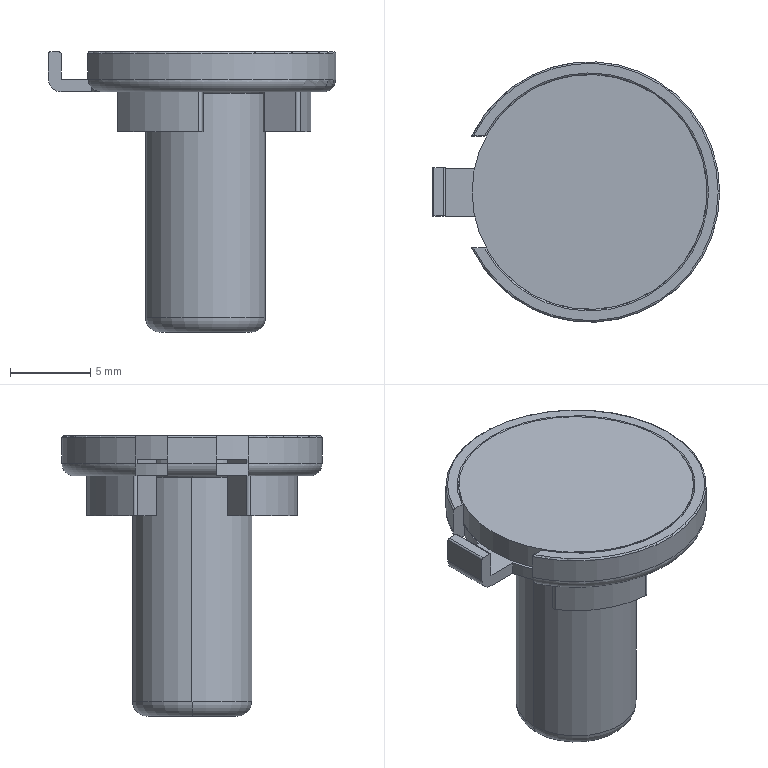NC program | NX | posted with a generic post | part box 17.958 x 16.273 x 17.5 mm
Lines 1 to 900 of 9718:
N10 G17 G21 G94 G90
(ZLEVEL_PROFILE_COPY , TOOL : D4)
N12 T04 M6
N14 G54
N16 G17 G0 G90 X-5.215 Y0.746 S6500 M3
N18 G43 Z10.55 H4
N20 Z-0.077
N22 G94 G1 X-5.509 Y1.253 F1800.
N24 G3 X-5.855 Y1.452 R0.4
N26 G1 X-6.414 Y1.451
N28 X-6.45 Y1.45
N30 X-6.971
N32 Y0.
N34 X-6.972 Y-0.018
N36 Y-1.45
N38 X-6.29
N40 X-5.873 Y-1.452
N42 G3 X-5.526 Y-1.253 R0.4
N44 G1 X-5.228 Y-0.743
N46 G0 X-5.215 Y0.746 Z-0.155
N48 G1 X-5.509 Y1.253
N50 G3 X-5.855 Y1.452 R0.4
N52 G1 X-6.414 Y1.451
N54 X-6.448 Y1.45
N56 X-6.971
N58 Y-1.45
N60 X-6.448
N62 X-6.255 Y-1.459
N64 X-6.246 Y-1.455
N66 X-6.219 Y-1.439
N68 X-6.188 Y-1.445
N70 X-6.168 Y-1.469
N72 X-6.148 Y-1.451
N74 X-5.855 Y-1.452
N76 G3 X-5.509 Y-1.253 R0.4
N78 G1 X-5.215 Y-0.746
N80 G0 Y0.746 Z-0.232
N82 G1 X-5.509 Y1.253
N84 G3 X-5.855 Y1.452 R0.4
N86 G1 X-6.414 Y1.451
N88 X-6.448 Y1.45
N90 X-6.971
N92 Y-1.45
N94 X-6.448
N96 X-6.255 Y-1.459
N98 X-6.246 Y-1.455
N100 X-6.219 Y-1.439
N102 X-6.188 Y-1.445
N104 X-6.168 Y-1.469
N106 X-6.148 Y-1.451
N108 X-5.855 Y-1.452
N110 G3 X-5.509 Y-1.253 R0.4
N112 G1 X-5.215 Y-0.746
N114 G0 Y0.746 Z-0.309
N116 G1 X-5.509 Y1.253
N118 G3 X-5.855 Y1.452 R0.4
N120 G1 X-6.414 Y1.451
N122 X-6.448 Y1.45
N124 X-6.971
N126 Y-1.45
N128 X-6.448
N130 X-6.255 Y-1.459
N132 X-6.246 Y-1.455
N134 X-6.219 Y-1.439
N136 X-6.188 Y-1.445
N138 X-6.168 Y-1.469
N140 X-6.148 Y-1.451
N142 X-5.855 Y-1.452
N144 G3 X-5.509 Y-1.253 R0.4
N146 G1 X-5.215 Y-0.746
N148 G0 Y0.746 Z-0.386
N150 G1 X-5.509 Y1.253
N152 G3 X-5.855 Y1.452 R0.4
N154 G1 X-6.414 Y1.451
N156 X-6.448 Y1.45
N158 X-6.971
N160 Y-1.45
N162 X-6.448 Y-1.449
N164 X-6.255 Y-1.459
N166 X-6.246 Y-1.455
N168 X-6.219 Y-1.439
N170 X-6.188 Y-1.445
N172 X-6.168 Y-1.469
N174 X-6.148 Y-1.451
N176 X-5.855 Y-1.452
N178 G3 X-5.509 Y-1.252 R0.4
N180 G1 X-5.215 Y-0.746
N182 G0 Y0.746 Z-0.464
N184 G1 X-5.509 Y1.253
N186 G3 X-5.855 Y1.452 R0.4
N188 G1 X-6.414 Y1.451
N190 X-6.448 Y1.45
N192 X-6.971
N194 Y-1.45
N196 X-6.448 Y-1.449
N198 X-6.255 Y-1.459
N200 X-6.246 Y-1.455
N202 X-6.219 Y-1.439
N204 X-6.188 Y-1.445
N206 X-6.168 Y-1.469
N208 X-6.148 Y-1.451
N210 X-5.855 Y-1.452
N212 G3 X-5.509 Y-1.252 R0.4
N214 G1 X-5.215 Y-0.745
N216 G0 Y0.746 Z-0.541
N218 G1 X-5.509 Y1.252
N220 G3 X-5.855 Y1.452 R0.4
N222 G1 X-6.414 Y1.451
N224 X-6.448 Y1.45
N226 X-6.971
N228 Y-1.45
N230 X-6.448 Y-1.449
N232 X-6.255 Y-1.459
N234 X-6.246 Y-1.455
N236 X-6.219 Y-1.439
N238 X-6.188 Y-1.445
N240 X-6.168 Y-1.469
N242 X-6.148 Y-1.451
N244 X-5.855 Y-1.452
N246 G3 X-5.509 Y-1.252 R0.4
N248 G1 X-5.215 Y-0.745
N250 G0 Y0.745 Z-0.618
N252 G1 X-5.509 Y1.252
N254 G3 X-5.855 Y1.452 R0.4
N256 G1 X-6.414 Y1.451
N258 X-6.448 Y1.45
N260 X-6.971
N262 Y-1.45
N264 X-6.448 Y-1.449
N266 X-6.255 Y-1.459
N268 X-6.246 Y-1.455
N270 X-6.219 Y-1.439
N272 X-6.188 Y-1.445
N274 X-6.168 Y-1.469
N276 X-6.148 Y-1.451
N278 X-5.855 Y-1.452
N280 G3 X-5.509 Y-1.252 R0.4
N282 G1 X-5.215 Y-0.745
N284 G0 Y0.745 Z-0.695
N286 G1 X-5.509 Y1.252
N288 G3 X-5.855 Y1.452 R0.4
N290 G1 X-6.414 Y1.451
N292 X-6.448 Y1.45
N294 X-6.971
N296 Y-1.45
N298 X-6.448 Y-1.449
N300 X-6.255 Y-1.459
N302 X-6.246 Y-1.455
N304 X-6.219 Y-1.439
N306 X-6.188 Y-1.444
N308 X-6.168 Y-1.469
N310 X-6.148 Y-1.451
N312 X-5.855 Y-1.452
N314 G3 X-5.509 Y-1.252 R0.4
N316 G1 X-5.215 Y-0.745
N318 G0 Y0.745 Z-0.773
N320 G1 X-5.509 Y1.252
N322 G3 X-5.855 Y1.452 R0.4
N324 G1 X-6.414 Y1.451
N326 X-6.448 Y1.45
N328 X-6.971
N330 Y-1.45
N332 X-6.448 Y-1.449
N334 X-6.255 Y-1.459
N336 X-6.246 Y-1.455
N338 X-6.219 Y-1.439
N340 X-6.188 Y-1.444
N342 X-6.168 Y-1.469
N344 X-6.148 Y-1.451
N346 X-5.855 Y-1.452
N348 G3 X-5.509 Y-1.252 R0.4
N350 G1 X-5.215 Y-0.745
N352 G0 Y0.745 Z-0.85
N354 G1 X-5.509 Y1.252
N356 G3 X-5.855 Y1.451 R0.4
N358 G1 X-6.414
N360 X-6.448 Y1.45
N362 X-6.971
N364 Y-1.45
N366 X-6.448 Y-1.449
N368 X-6.255 Y-1.459
N370 X-6.246 Y-1.455
N372 X-6.219 Y-1.439
N374 X-6.188 Y-1.444
N376 X-6.168 Y-1.469
N378 X-6.148 Y-1.451
N380 X-5.855
N382 G3 X-5.509 Y-1.252 R0.4
N384 G1 X-5.215 Y-0.745
N386 G0 Y0.745 Z-0.927
N388 G1 X-5.509 Y1.252
N390 G3 X-5.855 Y1.451 R0.4
N392 G1 X-6.414 Y1.45
N394 X-6.448
N396 X-6.971
N398 Y-1.45
N400 X-6.448 Y-1.449
N402 X-6.255 Y-1.459
N404 X-6.246 Y-1.455
N406 X-6.219 Y-1.438
N408 X-6.188 Y-1.444
N410 X-6.168 Y-1.469
N412 X-6.148 Y-1.45
N414 X-5.855 Y-1.451
N416 G3 X-5.509 Y-1.252 R0.4
N418 G1 X-5.216 Y-0.745
N420 G0 X-5.215 Y0.745 Z-1.005
N422 G1 X-5.509 Y1.252
N424 G3 X-5.855 Y1.451 R0.4
N426 G1 X-6.414 Y1.45
N428 X-6.448
N430 X-6.971
N432 Y-1.45
N434 X-6.464
N436 X-6.448 Y-1.449
N438 X-6.255 Y-1.459
N440 X-6.246 Y-1.455
N442 X-6.219 Y-1.438
N444 X-6.188 Y-1.444
N446 X-6.168 Y-1.469
N448 X-6.148 Y-1.45
N450 X-5.855 Y-1.451
N452 G3 X-5.509 Y-1.252 R0.4
N454 G1 X-5.216 Y-0.744
N456 G0 X-5.214 Y0.745 Z-1.082
N458 G1 X-5.509 Y1.252
N460 G3 X-5.855 Y1.451 R0.4
N462 G1 X-6.448 Y1.45
N464 X-6.971
N466 Y-1.45
N468 X-6.464
N470 X-6.448 Y-1.449
N472 X-6.255 Y-1.459
N474 X-6.246 Y-1.455
N476 X-6.219 Y-1.438
N478 X-6.188 Y-1.444
N480 X-6.168 Y-1.469
N482 X-6.148 Y-1.45
N484 X-5.855 Y-1.451
N486 G3 X-5.509 Y-1.251 R0.4
N488 G1 X-5.216 Y-0.744
N490 G0 X-5.214 Y0.744 Z-1.159
N492 G1 X-5.509 Y1.252
N494 G3 X-5.855 Y1.451 R0.4
N496 G1 X-6.448 Y1.45
N498 X-6.971
N500 Y-1.45
N502 X-6.464
N504 X-6.448 Y-1.449
N506 X-6.255 Y-1.459
N508 X-6.246 Y-1.455
N510 X-6.219 Y-1.438
N512 X-6.188 Y-1.444
N514 X-6.168 Y-1.469
N516 X-6.148 Y-1.45
N518 X-5.855 Y-1.451
N520 G3 X-5.509 Y-1.251 R0.4
N522 G1 X-5.216 Y-0.744
N524 G0 X-5.205 Y0.728 Z-1.236
N526 G1 X-5.509 Y1.251
N528 G3 X-5.855 Y1.451 R0.4
N530 G1 X-6.448 Y1.45
N532 X-6.971
N534 Y-1.45
N536 X-6.464
N538 X-6.448 Y-1.449
N540 X-6.255 Y-1.459
N542 X-6.246 Y-1.455
N544 X-6.219 Y-1.438
N546 X-6.188 Y-1.444
N548 X-6.168 Y-1.469
N550 X-6.148 Y-1.45
N552 X-5.855 Y-1.451
N554 G3 X-5.508 Y-1.252 R0.4
N556 G1 X-5.204 Y-0.728
N558 G0 X-5.206 Y0.728 Z-1.314
N560 G1 X-5.509 Y1.251
N562 G3 X-5.855 Y1.451 R0.4
N564 G1 X-6.448 Y1.45
N566 X-6.971
N568 Y-1.45
N570 X-6.464
N572 X-6.448 Y-1.449
N574 X-6.255 Y-1.459
N576 X-6.246 Y-1.455
N578 X-6.219 Y-1.438
N580 X-6.187 Y-1.444
N582 X-6.168 Y-1.469
N584 X-6.148 Y-1.45
N586 X-5.855 Y-1.451
N588 G3 X-5.509 Y-1.252 R0.4
N590 G1 X-5.205 Y-0.728
N592 G0 X-5.206 Y0.727 Z-1.391
N594 G1 X-5.509 Y1.251
N596 G3 X-5.855 Y1.451 R0.4
N598 G1 X-6.448 Y1.45
N600 X-6.971
N602 Y-1.45
N604 X-6.464
N606 X-6.448 Y-1.449
N608 X-6.255 Y-1.459
N610 X-6.246 Y-1.455
N612 X-6.219 Y-1.438
N614 X-6.187 Y-1.444
N616 X-6.168 Y-1.469
N618 X-6.148 Y-1.45
N620 X-5.855 Y-1.451
N622 G3 X-5.509 Y-1.251 R0.4
N624 G1 X-5.205 Y-0.727
N626 G0 X-5.206 Y0.727 Z-1.468
N628 G1 X-5.509 Y1.251
N630 G3 X-5.855 Y1.45 R0.4
N632 G1 X-6.448
N634 X-6.971
N636 Y-1.45
N638 X-6.464
N640 X-6.448 Y-1.449
N642 X-6.255 Y-1.459
N644 X-6.246 Y-1.455
N646 X-6.219 Y-1.438
N648 X-6.187 Y-1.444
N650 X-6.168 Y-1.469
N652 X-6.148 Y-1.45
N654 X-5.855
N656 G3 X-5.509 Y-1.251 R0.4
N658 G1 X-5.205 Y-0.727
N660 G0 X-5.207 Y0.727 Z-1.545
N662 G1 X-5.509 Y1.25
N664 G3 X-5.855 Y1.45 R0.4
N666 G1 X-6.448
N668 X-6.971
N670 Y-1.45
N672 X-6.464
N674 X-6.448 Y-1.448
N676 X-6.255 Y-1.459
N678 X-6.246 Y-1.454
N680 X-6.219 Y-1.438
N682 X-6.187 Y-1.444
N684 X-6.168 Y-1.469
N686 X-6.148 Y-1.45
N688 X-5.855
N690 G3 X-5.509 Y-1.25 R0.4
N692 G1 X-5.206 Y-0.727
N694 G0 X-5.215 Y0.725 Z-1.623
N696 G1 X-5.518 Y1.25
N698 G3 X-5.864 Y1.45 R0.4
N700 G1 X-6.448
N702 X-6.971
N704 Y-1.45
N706 X-6.464
N708 X-6.448 Y-1.448
N710 X-6.255 Y-1.459
N712 X-6.246 Y-1.454
N714 X-6.219 Y-1.438
N716 X-6.187 Y-1.444
N718 X-6.168 Y-1.469
N720 X-6.169 Y-1.448
N722 X-6.148 Y-1.45
N724 X-5.864
N726 G3 X-5.518 Y-1.25 R0.4
N728 G1 X-5.214 Y-0.725
N730 G0 X-5.215 Y0.724 Z-1.7
N732 G1 X-5.518 Y1.25
N734 G3 X-5.864 Y1.45 R0.4
N736 G1 X-6.448
N738 X-6.971
N740 Y-1.45
N742 X-6.464
N744 X-6.448 Y-1.448
N746 X-6.255 Y-1.459
N748 X-6.246 Y-1.454
N750 X-6.219 Y-1.438
N752 X-6.187 Y-1.444
N754 X-6.168 Y-1.469
N756 X-6.169 Y-1.448
N758 X-6.148 Y-1.45
N760 X-5.864
N762 G3 X-5.518 Y-1.25 R0.4
N764 G1 X-5.215 Y-0.724
N766 G0 Z10.55
(ZLEVEL_PROFILE_COPY_COPY_1 , TOOL : D4)
N768 X-5.217 Y0.775
N770 Z10.5
N772 Z-1.7
N774 G1 X-5.52 Y1.3 F1000.
N776 G3 X-5.867 Y1.5 R0.4
N778 G1 X-6.448
N780 X-7.021
N782 Y-1.5
N784 X-6.448
N786 X-5.867
N788 G3 X-5.52 Y-1.3 R0.4
N790 G1 X-5.217 Y-0.775
N792 G0 Z10.5
(ZLEVEL_PROFILE_COPY_COPY , TOOL : D4)
N794 Z10.55
N796 X-12.671 Y-0.699
N798 Z-0.078
N800 G1 X-12.071 Y-0.352 F1800.
N802 G3 X-11.871 Y-0.006 R0.4
N804 G1 Y1.494
N806 G2 X-9.815 Y3.55 R2.056
N808 G1 X-9.395
N810 X-9.393 Y3.595
N812 G2 X-9.19 Y4.394 R2.155
N814 X-3.659 Y9.507 R10.196
N816 G1 X-3.633 Y9.515
N818 G2 X-2.792 Y9.795 R8.817
N820 X2.815 Y9.79 R10.159
N822 X9.514 Y3.638 R10.187
N824 G1 X9.587 Y3.44
N826 G2 X9.793 Y2.798 R8.184
N828 X9.795 Y-2.798 R10.168
N830 G1 X9.793
N832 X9.791 Y-2.807
N834 G2 X9.506 Y-3.656 R9.385
N836 X3.076 Y-9.709 R10.173
N838 G1 X2.797 Y-9.794
N840 G2 X-2.81 Y-9.79 R10.206
N842 X-3.658 Y-9.505 R9.792
N844 X-9.198 Y-4.375 R10.179
N846 X-9.393 Y-3.549 R2.056
N848 G1 X-9.4 Y-3.55
N850 X-9.829
N852 G2 X-11.871 Y-1.506 R2.043
N854 G1 Y-0.006
N856 G3 X-12.071 Y0.34 R0.4
N858 G1 X-12.671 Y0.687
N860 G0 Y-0.699 Z-0.156
N862 G1 X-12.071 Y-0.352
N864 G3 X-11.871 Y-0.006 R0.4
N866 G1 Y1.5
N868 G2 X-9.821 Y3.55 R2.05
N870 G1 X-9.395
N872 G2 X-9.196 Y4.382 R2.05
N874 X-9.196 Y-4.382 R-10.187
N876 X-9.395 Y-3.55 R2.05
N878 G1 X-9.821
N880 G2 X-11.871 Y-1.5 R2.05
N882 G1 Y-0.006
N884 G3 X-12.071 Y0.34 R0.4
N886 G1 X-12.671 Y0.687
N888 G0 Y-0.699 Z-0.234
N890 G1 X-12.071 Y-0.352
N892 G3 X-11.871 Y-0.006 R0.4
N894 G1 Y1.5
N896 G2 X-9.821 Y3.55 R2.05
N898 G1 X-9.395
N900 G2 X-9.196 Y4.382 R2.05
N902 X-9.196 Y-4.382 R-10.187
N904 X-9.395 Y-3.55 R2.05
N906 G1 X-9.821
N908 G2 X-11.871 Y-1.5 R2.05
N910 G1 Y-0.006
N912 G3 X-12.071 Y0.34 R0.4
N914 G1 X-12.671 Y0.687
N916 G0 Y-0.699 Z-0.313
N918 G1 X-12.071 Y-0.352
N920 G3 X-11.871 Y-0.006 R0.4
N922 G1 Y1.5
N924 G2 X-9.821 Y3.55 R2.05
N926 G1 X-9.395
N928 G2 X-9.196 Y4.382 R2.05
N930 X-9.196 Y-4.382 R-10.187
N932 X-9.395 Y-3.55 R2.05
N934 G1 X-9.821
N936 G2 X-11.871 Y-1.5 R2.05
N938 G1 Y-0.006
N940 G3 X-12.071 Y0.34 R0.4
N942 G1 X-12.671 Y0.687
N944 G0 Y-0.699 Z-0.391
N946 G1 X-12.071 Y-0.352
N948 G3 X-11.871 Y-0.006 R0.4
N950 G1 Y1.5
N952 G2 X-9.821 Y3.55 R2.05
N954 G1 X-9.395
N956 G2 X-9.196 Y4.382 R2.05
N958 X-9.196 Y-4.382 R-10.187
N960 X-9.395 Y-3.55 R2.05
N962 G1 X-9.821
N964 G2 X-11.871 Y-1.5 R2.05
N966 G1 Y-0.006
N968 G3 X-12.071 Y0.34 R0.4
N970 G1 X-12.671 Y0.687
N972 G0 Y-0.699 Z-0.469
N974 G1 X-12.071 Y-0.352
N976 G3 X-11.871 Y-0.006 R0.4
N978 G1 Y1.5
N980 G2 X-9.821 Y3.55 R2.05
N982 G1 X-9.395
N984 G2 X-9.196 Y4.382 R2.05
N986 X-9.196 Y-4.382 R-10.187
N988 X-9.395 Y-3.55 R2.05
N990 G1 X-9.821
N992 G2 X-11.871 Y-1.5 R2.05
N994 G1 Y-0.006
N996 G3 X-12.071 Y0.34 R0.4
N998 G1 X-12.671 Y0.687
N1000 G0 Y-0.699 Z-0.547
N1002 G1 X-12.071 Y-0.352
N1004 G3 X-11.871 Y-0.006 R0.4
N1006 G1 Y1.5
N1008 G2 X-9.821 Y3.55 R2.05
N1010 G1 X-9.395
N1012 G2 X-9.196 Y4.382 R2.05
N1014 X-9.196 Y-4.382 R-10.187
N1016 X-9.395 Y-3.55 R2.05
N1018 G1 X-9.821
N1020 G2 X-11.871 Y-1.5 R2.05
N1022 G1 Y-0.006
N1024 G3 X-12.071 Y0.34 R0.4
N1026 G1 X-12.671 Y0.687
N1028 G0 Y-0.699 Z-0.625
N1030 G1 X-12.071 Y-0.352
N1032 G3 X-11.871 Y-0.006 R0.4
N1034 G1 Y1.5
N1036 G2 X-9.821 Y3.55 R2.05
N1038 G1 X-9.395
N1040 G2 X-9.196 Y4.382 R2.05
N1042 X-9.196 Y-4.382 R-10.187
N1044 X-9.395 Y-3.55 R2.05
N1046 G1 X-9.821
N1048 G2 X-11.871 Y-1.5 R2.05
N1050 G1 Y-0.006
N1052 G3 X-12.071 Y0.34 R0.4
N1054 G1 X-12.671 Y0.687
N1056 G0 Y-0.699 Z-0.703
N1058 G1 X-12.071 Y-0.352
N1060 G3 X-11.871 Y-0.006 R0.4
N1062 G1 Y1.5
N1064 G2 X-9.821 Y3.55 R2.05
N1066 G1 X-9.395
N1068 G2 X-9.196 Y4.382 R2.05
N1070 X-9.196 Y-4.382 R-10.187
N1072 X-9.395 Y-3.55 R2.05
N1074 G1 X-9.821
N1076 G2 X-11.871 Y-1.5 R2.05
N1078 G1 Y-0.006
N1080 G3 X-12.071 Y0.34 R0.4
N1082 G1 X-12.671 Y0.687
N1084 G0 Y-0.699 Z-0.781
N1086 G1 X-12.071 Y-0.352
N1088 G3 X-11.871 Y-0.006 R0.4
N1090 G1 Y1.5
N1092 G2 X-9.821 Y3.55 R2.05
N1094 G1 X-9.395
N1096 G2 X-9.196 Y4.382 R2.05
N1098 X-9.196 Y-4.382 R-10.187
N1100 X-9.395 Y-3.55 R2.05
N1102 G1 X-9.821
N1104 G2 X-11.871 Y-1.5 R2.05
N1106 G1 Y-0.006
N1108 G3 X-12.071 Y0.34 R0.4
N1110 G1 X-12.671 Y0.687
N1112 G0 Y-0.699 Z-0.859
N1114 G1 X-12.071 Y-0.352
N1116 G3 X-11.871 Y-0.006 R0.4
N1118 G1 Y1.5
N1120 G2 X-9.821 Y3.55 R2.05
N1122 G1 X-9.395
N1124 G2 X-9.196 Y4.382 R2.05
N1126 X-9.196 Y-4.382 R-10.187
N1128 X-9.395 Y-3.55 R2.05
N1130 G1 X-9.821
N1132 G2 X-11.871 Y-1.5 R2.05
N1134 G1 Y-0.006
N1136 G3 X-12.071 Y0.34 R0.4
N1138 G1 X-12.671 Y0.687
N1140 G0 Y-0.699 Z-0.938
N1142 G1 X-12.071 Y-0.352
N1144 G3 X-11.871 Y-0.006 R0.4
N1146 G1 Y1.5
N1148 G2 X-9.821 Y3.55 R2.05
N1150 G1 X-9.395
N1152 G2 X-9.196 Y4.382 R2.05
N1154 X-9.196 Y-4.382 R-10.187
N1156 X-9.395 Y-3.55 R2.05
N1158 G1 X-9.821
N1160 G2 X-11.871 Y-1.5 R2.05
N1162 G1 Y-0.006
N1164 G3 X-12.071 Y0.34 R0.4
N1166 G1 X-12.671 Y0.687
N1168 G0 Y-0.699 Z-1.016
N1170 G1 X-12.071 Y-0.352
N1172 G3 X-11.871 Y-0.006 R0.4
N1174 G1 Y1.5
N1176 G2 X-9.821 Y3.55 R2.05
N1178 G1 X-9.395
N1180 G2 X-9.196 Y4.382 R2.05
N1182 X-9.196 Y-4.382 R-10.187
N1184 X-9.395 Y-3.55 R2.05
N1186 G1 X-9.821
N1188 G2 X-11.871 Y-1.5 R2.05
N1190 G1 Y-0.006
N1192 G3 X-12.071 Y0.34 R0.4
N1194 G1 X-12.671 Y0.687
N1196 G0 Y-0.699 Z-1.094
N1198 G1 X-12.071 Y-0.352
N1200 G3 X-11.871 Y-0.006 R0.4
N1202 G1 Y1.5
N1204 G2 X-9.821 Y3.55 R2.05
N1206 G1 X-9.395
N1208 G2 X-9.196 Y4.382 R2.05
N1210 X-9.196 Y-4.382 R-10.187
N1212 X-9.395 Y-3.55 R2.05
N1214 G1 X-9.821
N1216 G2 X-11.871 Y-1.5 R2.05
N1218 G1 Y-0.006
N1220 G3 X-12.071 Y0.34 R0.4
N1222 G1 X-12.671 Y0.687
N1224 G0 Y-0.699 Z-1.172
N1226 G1 X-12.071 Y-0.352
N1228 G3 X-11.871 Y-0.006 R0.4
N1230 G1 Y1.5
N1232 G2 X-9.821 Y3.55 R2.05
N1234 G1 X-9.395
N1236 G2 X-9.196 Y4.382 R2.05
N1238 X-9.196 Y-4.382 R-10.187
N1240 X-9.395 Y-3.55 R2.05
N1242 G1 X-9.821
N1244 G2 X-11.871 Y-1.5 R2.05
N1246 G1 Y-0.006
N1248 G3 X-12.071 Y0.34 R0.4
N1250 G1 X-12.671 Y0.687
N1252 G0 Y-0.699 Z-1.25
N1254 G1 X-12.071 Y-0.352
N1256 G3 X-11.871 Y-0.006 R0.4
N1258 G1 Y1.5
N1260 G2 X-9.821 Y3.55 R2.05
N1262 G1 X-9.395
N1264 G2 X-9.196 Y4.382 R2.05
N1266 X-9.196 Y-4.382 R-10.187
N1268 X-9.395 Y-3.55 R2.05
N1270 G1 X-9.821
N1272 G2 X-11.871 Y-1.5 R2.05
N1274 G1 Y-0.006
N1276 G3 X-12.071 Y0.34 R0.4
N1278 G1 X-12.671 Y0.687
N1280 G0 Y-0.699 Z-1.328
N1282 G1 X-12.071 Y-0.352
N1284 G3 X-11.871 Y-0.006 R0.4
N1286 G1 Y1.5
N1288 G2 X-9.821 Y3.55 R2.05
N1290 G1 X-9.395
N1292 G2 X-9.196 Y4.382 R2.05
N1294 X-9.196 Y-4.382 R-10.187
N1296 X-9.395 Y-3.55 R2.05
N1298 G1 X-9.821
N1300 G2 X-11.871 Y-1.5 R2.05
N1302 G1 Y-0.006
N1304 G3 X-12.071 Y0.34 R0.4
N1306 G1 X-12.671 Y0.687
N1308 G0 Y-0.699 Z-1.406
N1310 G1 X-12.071 Y-0.352
N1312 G3 X-11.871 Y-0.006 R0.4
N1314 G1 Y1.5
N1316 G2 X-9.821 Y3.55 R2.05
N1318 G1 X-9.395
N1320 G2 X-9.196 Y4.382 R2.05
N1322 X-9.196 Y-4.382 R-10.187
N1324 X-9.395 Y-3.55 R2.05
N1326 G1 X-9.821
N1328 G2 X-11.871 Y-1.5 R2.05
N1330 G1 Y-0.006
N1332 G3 X-12.071 Y0.34 R0.4
N1334 G1 X-12.671 Y0.687
N1336 G0 Y-0.699 Z-1.484
N1338 G1 X-12.071 Y-0.352
N1340 G3 X-11.871 Y-0.006 R0.4
N1342 G1 Y1.5
N1344 G2 X-9.821 Y3.55 R2.05
N1346 G1 X-9.395
N1348 G2 X-9.196 Y4.382 R2.05
N1350 X-9.196 Y-4.382 R-10.187
N1352 X-9.395 Y-3.55 R2.05
N1354 G1 X-9.821
N1356 G2 X-11.871 Y-1.5 R2.05
N1358 G1 Y-0.006
N1360 G3 X-12.071 Y0.34 R0.4
N1362 G1 X-12.671 Y0.687
N1364 G0 Y-0.699 Z-1.563
N1366 G1 X-12.071 Y-0.352
N1368 G3 X-11.871 Y-0.006 R0.4
N1370 G1 Y1.5
N1372 G2 X-9.821 Y3.55 R2.05
N1374 G1 X-9.395
N1376 G2 X-9.196 Y4.382 R2.05
N1378 X-9.196 Y-4.382 R-10.187
N1380 X-9.395 Y-3.55 R2.05
N1382 G1 X-9.821
N1384 G2 X-11.871 Y-1.5 R2.05
N1386 G1 Y-0.006
N1388 G3 X-12.071 Y0.34 R0.4
N1390 G1 X-12.671 Y0.687
N1392 G0 Y-0.699 Z-1.641
N1394 G1 X-12.071 Y-0.352
N1396 G3 X-11.871 Y-0.006 R0.4
N1398 G1 Y1.5
N1400 G2 X-9.821 Y3.55 R2.05
N1402 G1 X-9.395
N1404 G2 X-9.196 Y4.382 R2.05
N1406 X-9.196 Y-4.382 R-10.187
N1408 X-9.395 Y-3.55 R2.05
N1410 G1 X-9.821
N1412 G2 X-11.871 Y-1.5 R2.05
N1414 G1 Y-0.006
N1416 G3 X-12.071 Y0.34 R0.4
N1418 G1 X-12.671 Y0.687
N1420 G0 Y-0.699 Z-1.719
N1422 G1 X-12.071 Y-0.352
N1424 G3 X-11.871 Y-0.006 R0.4
N1426 G1 Y1.5
N1428 G2 X-9.821 Y3.55 R2.05
N1430 G1 X-9.395
N1432 G2 X-9.196 Y4.382 R2.05
N1434 X-9.196 Y-4.382 R-10.187
N1436 X-9.395 Y-3.55 R2.05
N1438 G1 X-9.821
N1440 G2 X-11.871 Y-1.5 R2.05
N1442 G1 Y-0.006
N1444 G3 X-12.071 Y0.34 R0.4
N1446 G1 X-12.671 Y0.687
N1448 G0 Y-0.699 Z-1.797
N1450 G1 X-12.071 Y-0.352
N1452 G3 X-11.871 Y-0.006 R0.4
N1454 G1 Y1.5
N1456 G2 X-9.821 Y3.55 R2.05
N1458 G1 X-9.395
N1460 G2 X-9.196 Y4.382 R2.05
N1462 X-9.196 Y-4.382 R-10.187
N1464 X-9.395 Y-3.55 R2.05
N1466 G1 X-9.821
N1468 G2 X-11.871 Y-1.5 R2.05
N1470 G1 Y-0.006
N1472 G3 X-12.071 Y0.34 R0.4
N1474 G1 X-12.671 Y0.687
N1476 G0 Y-0.699 Z-1.875
N1478 G1 X-12.071 Y-0.352
N1480 G3 X-11.871 Y-0.006 R0.4
N1482 G1 Y1.5
N1484 G2 X-9.821 Y3.55 R2.05
N1486 G1 X-9.395
N1488 G2 X-9.196 Y4.382 R2.05
N1490 X-9.196 Y-4.382 R-10.187
N1492 X-9.395 Y-3.55 R2.05
N1494 G1 X-9.821
N1496 G2 X-11.871 Y-1.5 R2.05
N1498 G1 Y-0.006
N1500 G3 X-12.071 Y0.34 R0.4
N1502 G1 X-12.671 Y0.687
N1504 G0 Y-0.699 Z-1.953
N1506 G1 X-12.071 Y-0.352
N1508 G3 X-11.871 Y-0.006 R0.4
N1510 G1 Y1.5
N1512 G2 X-9.821 Y3.55 R2.05
N1514 G1 X-9.395
N1516 G2 X-9.196 Y4.382 R2.05
N1518 X-9.196 Y-4.382 R-10.187
N1520 X-9.395 Y-3.55 R2.05
N1522 G1 X-9.821
N1524 G2 X-11.871 Y-1.5 R2.05
N1526 G1 Y-0.006
N1528 G3 X-12.071 Y0.34 R0.4
N1530 G1 X-12.671 Y0.687
N1532 G0 Y-0.699 Z-2.031
N1534 G1 X-12.071 Y-0.352
N1536 G3 X-11.871 Y-0.006 R0.4
N1538 G1 Y1.5
N1540 G2 X-9.821 Y3.55 R2.05
N1542 G1 X-9.395
N1544 X-9.394 Y3.572
N1546 G2 X-9.196 Y4.382 R2.05
N1548 X-9.196 Y-4.382 R-10.187
N1550 X-9.395 Y-3.55 R2.05
N1552 G1 X-9.821
N1554 G2 X-11.871 Y-1.5 R2.05
N1556 G1 Y-0.006
N1558 G3 X-12.071 Y0.34 R0.4
N1560 G1 X-12.671 Y0.687
N1562 G0 Y-0.699 Z-2.109
N1564 G1 X-12.071 Y-0.352
N1566 G3 X-11.871 Y-0.006 R0.4
N1568 G1 Y1.5
N1570 G2 X-9.821 Y3.55 R2.05
N1572 G1 X-9.395
N1574 X-9.394 Y3.572
N1576 G2 X-9.196 Y4.382 R2.05
N1578 X-9.196 Y-4.382 R-10.187
N1580 X-9.395 Y-3.55 R2.05
N1582 G1 X-9.821
N1584 G2 X-11.871 Y-1.5 R2.05
N1586 G1 Y-0.006
N1588 G3 X-12.071 Y0.34 R0.4
N1590 G1 X-12.671 Y0.687
N1592 G0 Y-0.699 Z-2.188
N1594 G1 X-12.071 Y-0.352
N1596 G3 X-11.871 Y-0.006 R0.4
N1598 G1 Y1.5
N1600 G2 X-9.821 Y3.55 R2.05
N1602 G1 X-9.395
N1604 X-9.394 Y3.572
N1606 G2 X-9.196 Y4.382 R2.05
N1608 X-9.196 Y-4.382 R-10.187
N1610 X-9.395 Y-3.55 R2.05
N1612 G1 X-9.821
N1614 G2 X-11.871 Y-1.5 R2.05
N1616 G1 Y-0.006
N1618 G3 X-12.071 Y0.34 R0.4
N1620 G1 X-12.671 Y0.687
N1622 G0 Y-0.699 Z-2.266
N1624 G1 X-12.071 Y-0.352
N1626 G3 X-11.871 Y-0.006 R0.4
N1628 G1 Y1.5
N1630 G2 X-9.821 Y3.55 R2.05
N1632 G1 X-9.395
N1634 X-9.394 Y3.572
N1636 G2 X-9.196 Y4.382 R2.05
N1638 X-9.196 Y-4.382 R-10.187
N1640 X-9.395 Y-3.55 R2.05
N1642 G1 X-9.821
N1644 G2 X-11.871 Y-1.5 R2.05
N1646 G1 Y-0.006
N1648 G3 X-12.071 Y0.34 R0.4
N1650 G1 X-12.671 Y0.687
N1652 G0 Y-0.699 Z-2.344
N1654 G1 X-12.071 Y-0.352
N1656 G3 X-11.871 Y-0.006 R0.4
N1658 G1 Y1.5
N1660 G2 X-9.821 Y3.55 R2.05
N1662 G1 X-9.395
N1664 X-9.394 Y3.572
N1666 G2 X-9.196 Y4.382 R2.05
N1668 X-9.196 Y-4.382 R-10.187
N1670 X-9.395 Y-3.55 R2.05
N1672 G1 X-9.821
N1674 G2 X-11.871 Y-1.5 R2.05
N1676 G1 Y-0.006
N1678 G3 X-12.071 Y0.34 R0.4
N1680 G1 X-12.671 Y0.687
N1682 G0 Y-0.699 Z-2.422
N1684 G1 X-12.071 Y-0.352
N1686 G3 X-11.871 Y-0.006 R0.4
N1688 G1 Y1.5
N1690 G2 X-9.821 Y3.55 R2.05
N1692 G1 X-9.395
N1694 X-9.394 Y3.572
N1696 G2 X-9.196 Y4.382 R2.05
N1698 X-9.196 Y-4.382 R-10.187
N1700 X-9.395 Y-3.55 R2.05
N1702 G1 X-9.821
N1704 G2 X-11.871 Y-1.5 R2.05
N1706 G1 Y-0.006
N1708 G3 X-12.071 Y0.34 R0.4
N1710 G1 X-12.671 Y0.687
N1712 G0 Y-0.699 Z-2.5
N1714 G1 X-12.071 Y-0.352
N1716 G3 X-11.871 Y-0.006 R0.4
N1718 G1 Y1.5
N1720 G2 X-9.821 Y3.55 R2.05
N1722 G1 X-9.395
N1724 X-9.394 Y3.572
N1726 G2 X-9.196 Y4.382 R2.05
N1728 X-9.196 Y-4.382 R-10.187
N1730 X-9.395 Y-3.55 R2.05
N1732 G1 X-9.821
N1734 G2 X-11.871 Y-1.5 R2.05
N1736 G1 Y-0.006
N1738 G3 X-12.071 Y0.34 R0.4
N1740 G1 X-12.671 Y0.687
N1742 G0 Z10.55
(ZLEVEL_PROFILE_COPY_COPY_COPY , TOOL : D4)
N1744 X-12.621 Y-0.693
N1746 Z10.5
N1748 Z-2.5
N1750 G1 X-12.021 Y-0.346 F1000.
N1752 G3 X-11.821 Y0. R0.4
N1754 G1 Y1.5
N1756 G2 X-9.821 Y3.5 R2.
N1758 G1 X-9.345
N1760 Y3.525
N1762 G2 X-9.147 Y4.369 R2.
N1764 X-9.151 Y-4.36 R-10.137
N1766 X-9.345 Y-3.5 R2.
N1768 G1 X-9.821
N1770 G2 X-11.821 Y-1.5 R2.
N1772 G1 Y0.
N1774 G3 X-12.021 Y0.346 R0.4
N1776 G1 X-12.621 Y0.693
N1778 G0 Z10.5
N1780 M5